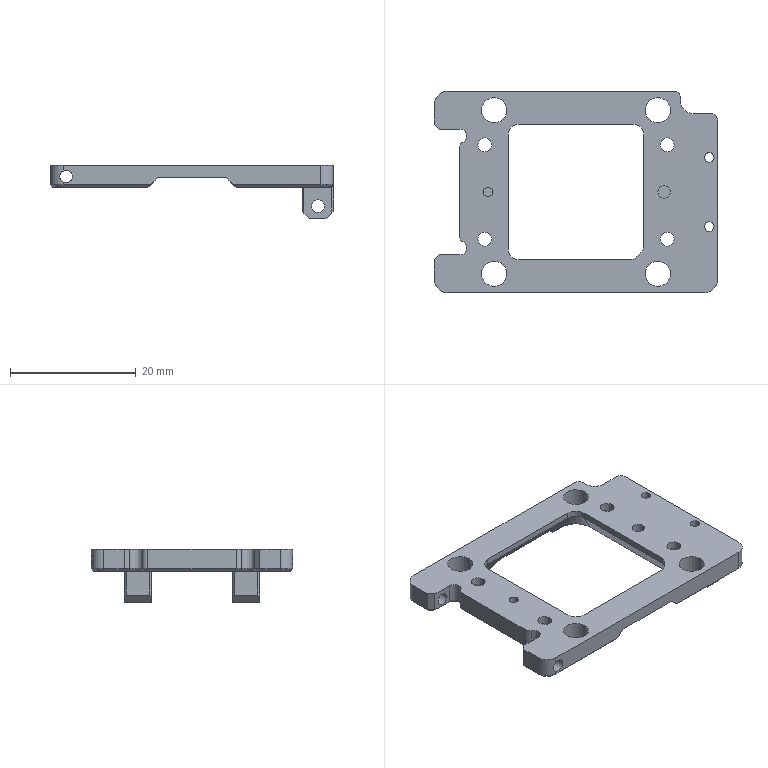NC program | NX | posted with a generic post | part box 45 x 32 x 8.5 mm
Lines 3037 to 3806 of 3806:
(CAVITY_MILL_COPY , TOOL : D1.5)
N6024 T19 M6
N6026 G54
N6028 G17 G0 G90 X-20.447 Y-8.95 B0. C0. S9500 M3
N6030 G43 Z30. H19
N6032 Z-0.146
N6034 G94 G3 X-19.733 Y-9.25 R1. F950.
N6036 G1 X-18.683
N6038 G2 X-18.483 Y-9.23 R0.76
N6040 G3 X-18.158 Y-8.974 R0.35
N6042 X-18.333 Y-8.592 R0.35
N6044 G2 X-19.055 Y-7.856 R1.75
N6046 G3 X-19.519 Y-7.41 R1.
N6048 G0 X-20.447 Y-8.95 Z-0.292
N6050 G3 X-19.733 Y-9.25 R1.
N6052 G1 X-18.683
N6054 G2 X-18.483 Y-9.23 R0.76
N6056 G3 X-18.158 Y-8.974 R0.35
N6058 X-18.333 Y-8.592 R0.35
N6060 G2 X-19.055 Y-7.856 R1.75
N6062 G3 X-19.519 Y-7.41 R1.
N6064 G0 X-20.447 Y-8.95 Z-0.438
N6066 G3 X-19.733 Y-9.25 R1.
N6068 G1 X-18.683
N6070 G2 X-18.483 Y-9.23 R0.76
N6072 G3 X-18.158 Y-8.974 R0.35
N6074 X-18.333 Y-8.592 R0.35
N6076 G2 X-19.055 Y-7.856 R1.75
N6078 G3 X-19.519 Y-7.41 R1.
N6080 G0 X-20.447 Y-8.95 Z-0.583
N6082 G3 X-19.733 Y-9.25 R1.
N6084 G1 X-18.683
N6086 G2 X-18.483 Y-9.23 R0.76
N6088 G3 X-18.158 Y-8.974 R0.35
N6090 X-18.333 Y-8.592 R0.35
N6092 G2 X-19.055 Y-7.856 R1.75
N6094 G3 X-19.519 Y-7.41 R1.
N6096 G0 X-20.447 Y-8.95 Z-0.729
N6098 G3 X-19.733 Y-9.25 R1.
N6100 G1 X-18.683
N6102 G2 X-18.483 Y-9.23 R0.76
N6104 G3 X-18.158 Y-8.974 R0.35
N6106 X-18.333 Y-8.592 R0.35
N6108 G2 X-19.055 Y-7.856 R1.75
N6110 G3 X-19.519 Y-7.41 R1.
N6112 G0 X-20.447 Y-8.95 Z-0.875
N6114 G3 X-19.733 Y-9.25 R1.
N6116 G1 X-18.683
N6118 G2 X-18.483 Y-9.23 R0.76
N6120 G3 X-18.158 Y-8.974 R0.35
N6122 X-18.333 Y-8.592 R0.35
N6124 G2 X-19.055 Y-7.856 R1.75
N6126 G3 X-19.519 Y-7.41 R1.
N6128 G0 X-20.447 Y-8.95 Z-1.021
N6130 G3 X-19.733 Y-9.25 R1.
N6132 G1 X-18.683
N6134 G2 X-18.483 Y-9.23 R0.76
N6136 G3 X-18.158 Y-8.974 R0.35
N6138 X-18.333 Y-8.592 R0.35
N6140 G2 X-19.055 Y-7.856 R1.75
N6142 G3 X-19.519 Y-7.41 R1.
N6144 G0 X-20.447 Y-8.95 Z-1.167
N6146 G3 X-19.733 Y-9.25 R1.
N6148 G1 X-18.683
N6150 G2 X-18.483 Y-9.23 R0.76
N6152 G3 X-18.158 Y-8.974 R0.35
N6154 X-18.333 Y-8.592 R0.35
N6156 G2 X-19.055 Y-7.856 R1.75
N6158 G3 X-19.519 Y-7.41 R1.
N6160 G0 X-20.447 Y-8.95 Z-1.313
N6162 G3 X-19.733 Y-9.25 R1.
N6164 G1 X-18.683
N6166 G2 X-18.483 Y-9.23 R0.76
N6168 G3 X-18.158 Y-8.974 R0.35
N6170 X-18.333 Y-8.592 R0.35
N6172 G2 X-19.055 Y-7.856 R1.75
N6174 G3 X-19.519 Y-7.41 R1.
N6176 G0 X-20.447 Y-8.95 Z-1.458
N6178 G3 X-19.733 Y-9.25 R1.
N6180 G1 X-18.683
N6182 G2 X-18.483 Y-9.23 R0.76
N6184 G3 X-18.158 Y-8.974 R0.35
N6186 X-18.333 Y-8.592 R0.35
N6188 G2 X-19.055 Y-7.856 R1.75
N6190 G3 X-19.519 Y-7.41 R1.
N6192 G0 X-20.447 Y-8.95 Z-1.604
N6194 G3 X-19.733 Y-9.25 R1.
N6196 G1 X-18.683
N6198 G2 X-18.483 Y-9.23 R0.76
N6200 G3 X-18.158 Y-8.974 R0.35
N6202 X-18.333 Y-8.592 R0.35
N6204 G2 X-19.055 Y-7.856 R1.75
N6206 G3 X-19.519 Y-7.41 R1.
N6208 G0 X-20.447 Y-8.95 Z-1.75
N6210 G3 X-19.733 Y-9.25 R1.
N6212 G1 X-18.683
N6214 G2 X-18.483 Y-9.23 R0.76
N6216 G3 X-18.158 Y-8.974 R0.35
N6218 X-18.333 Y-8.592 R0.35
N6220 G2 X-19.055 Y-7.856 R1.75
N6222 G3 X-19.519 Y-7.41 R1.
N6224 G0 X-20.447 Y-8.95 Z-1.896
N6226 G3 X-19.733 Y-9.25 R1.
N6228 G1 X-18.683
N6230 G2 X-18.483 Y-9.23 R0.76
N6232 G3 X-18.158 Y-8.974 R0.35
N6234 X-18.333 Y-8.592 R0.35
N6236 G2 X-19.055 Y-7.856 R1.75
N6238 G3 X-19.519 Y-7.41 R1.
N6240 G0 X-20.447 Y-8.95 Z-2.042
N6242 G3 X-19.733 Y-9.25 R1.
N6244 G1 X-18.683
N6246 G2 X-18.483 Y-9.23 R0.76
N6248 G3 X-18.158 Y-8.974 R0.35
N6250 X-18.333 Y-8.592 R0.35
N6252 G2 X-19.055 Y-7.856 R1.75
N6254 G3 X-19.519 Y-7.41 R1.
N6256 G0 X-20.447 Y-8.95 Z-2.188
N6258 G3 X-19.733 Y-9.25 R1.
N6260 G1 X-18.683
N6262 G2 X-18.483 Y-9.23 R0.76
N6264 G3 X-18.158 Y-8.974 R0.35
N6266 X-18.333 Y-8.592 R0.35
N6268 G2 X-19.055 Y-7.856 R1.75
N6270 G3 X-19.519 Y-7.41 R1.
N6272 G0 X-20.447 Y-8.95 Z-2.333
N6274 G3 X-19.733 Y-9.25 R1.
N6276 G1 X-18.683
N6278 G2 X-18.483 Y-9.23 R0.76
N6280 G3 X-18.158 Y-8.974 R0.35
N6282 X-18.333 Y-8.592 R0.35
N6284 G2 X-19.055 Y-7.856 R1.75
N6286 G3 X-19.519 Y-7.41 R1.
N6288 G0 X-20.447 Y-8.95 Z-2.479
N6290 G3 X-19.733 Y-9.25 R1.
N6292 G1 X-18.683
N6294 G2 X-18.483 Y-9.23 R0.76
N6296 G3 X-18.158 Y-8.974 R0.35
N6298 X-18.333 Y-8.592 R0.35
N6300 G2 X-19.055 Y-7.856 R1.75
N6302 G3 X-19.519 Y-7.41 R1.
N6304 G0 X-20.447 Y-8.95 Z-2.625
N6306 G3 X-19.733 Y-9.25 R1.
N6308 G1 X-18.683
N6310 G2 X-18.483 Y-9.23 R0.76
N6312 G3 X-18.158 Y-8.974 R0.35
N6314 X-18.333 Y-8.592 R0.35
N6316 G2 X-19.055 Y-7.856 R1.75
N6318 G3 X-19.519 Y-7.41 R1.
N6320 G0 X-20.447 Y-8.95 Z-2.771
N6322 G3 X-19.733 Y-9.25 R1.
N6324 G1 X-18.683
N6326 G2 X-18.483 Y-9.23 R0.76
N6328 G3 X-18.158 Y-8.974 R0.35
N6330 X-18.333 Y-8.592 R0.35
N6332 G2 X-19.055 Y-7.856 R1.75
N6334 G3 X-19.519 Y-7.41 R1.
N6336 G0 X-20.447 Y-8.95 Z-2.917
N6338 G3 X-19.733 Y-9.25 R1.
N6340 G1 X-18.683
N6342 G2 X-18.483 Y-9.23 R0.76
N6344 G3 X-18.158 Y-8.974 R0.35
N6346 X-18.333 Y-8.592 R0.35
N6348 G2 X-19.055 Y-7.856 R1.75
N6350 G3 X-19.519 Y-7.41 R1.
N6352 G0 X-20.447 Y-8.95 Z-3.063
N6354 G3 X-19.733 Y-9.25 R1.
N6356 G1 X-18.683
N6358 G2 X-18.483 Y-9.23 R0.76
N6360 G3 X-18.158 Y-8.974 R0.35
N6362 X-18.333 Y-8.592 R0.35
N6364 G2 X-19.055 Y-7.856 R1.75
N6366 G3 X-19.519 Y-7.41 R1.
N6368 G0 X-20.462 Y-8.95 Z-3.208
N6370 G3 X-19.748 Y-9.25 R1.
N6372 G1 X-18.683
N6374 G2 X-18.483 Y-9.23 R0.76
N6376 G3 X-18.158 Y-8.974 R0.35
N6378 X-18.333 Y-8.592 R0.35
N6380 G2 X-19.075 Y-7.816 R1.75
N6382 G3 X-19.527 Y-7.357 R1.
N6384 G0 X-20.462 Y-8.95 Z-3.354
N6386 G3 X-19.748 Y-9.25 R1.
N6388 G1 X-18.683
N6390 G2 X-18.483 Y-9.23 R0.76
N6392 G3 X-18.158 Y-8.974 R0.35
N6394 X-18.333 Y-8.592 R0.35
N6396 G2 X-19.075 Y-7.816 R1.75
N6398 G3 X-19.527 Y-7.357 R1.
N6400 G0 X-20.462 Y-8.95 Z-3.5
N6402 G3 X-19.748 Y-9.25 R1.
N6404 G1 X-18.683
N6406 G2 X-18.483 Y-9.23 R0.76
N6408 G3 X-18.158 Y-8.974 R0.35
N6410 X-18.333 Y-8.592 R0.35
N6412 G2 X-19.075 Y-7.816 R1.75
N6414 G3 X-19.527 Y-7.357 R1.
N6416 G0 Z30.
N6418 X-19.519 Y7.41
N6420 Z-0.146
N6422 G3 X-19.055 Y7.856 R1.
N6424 G2 X-18.333 Y8.592 R1.75
N6426 G3 X-18.158 Y8.974 R0.35
N6428 X-18.483 Y9.23 R0.331
N6430 G2 X-18.683 Y9.25 R0.76
N6432 G1 X-19.733
N6434 G3 X-20.447 Y8.95 R1.
N6436 G0 X-19.519 Y7.41 Z-0.292
N6438 G3 X-19.055 Y7.856 R1.
N6440 G2 X-18.333 Y8.592 R1.75
N6442 G3 X-18.158 Y8.974 R0.35
N6444 X-18.483 Y9.23 R0.331
N6446 G2 X-18.683 Y9.25 R0.76
N6448 G1 X-19.733
N6450 G3 X-20.447 Y8.95 R1.
N6452 G0 X-19.519 Y7.41 Z-0.438
N6454 G3 X-19.055 Y7.856 R1.
N6456 G2 X-18.333 Y8.592 R1.75
N6458 G3 X-18.158 Y8.974 R0.35
N6460 X-18.483 Y9.23 R0.331
N6462 G2 X-18.683 Y9.25 R0.76
N6464 G1 X-19.733
N6466 G3 X-20.447 Y8.95 R1.
N6468 G0 X-19.519 Y7.41 Z-0.583
N6470 G3 X-19.055 Y7.856 R1.
N6472 G2 X-18.333 Y8.592 R1.75
N6474 G3 X-18.158 Y8.974 R0.35
N6476 X-18.483 Y9.23 R0.331
N6478 G2 X-18.683 Y9.25 R0.76
N6480 G1 X-19.733
N6482 G3 X-20.447 Y8.95 R1.
N6484 G0 X-19.519 Y7.41 Z-0.729
N6486 G3 X-19.055 Y7.856 R1.
N6488 G2 X-18.333 Y8.592 R1.75
N6490 G3 X-18.158 Y8.974 R0.35
N6492 X-18.483 Y9.23 R0.331
N6494 G2 X-18.683 Y9.25 R0.76
N6496 G1 X-19.733
N6498 G3 X-20.447 Y8.95 R1.
N6500 G0 X-19.519 Y7.41 Z-0.875
N6502 G3 X-19.055 Y7.856 R1.
N6504 G2 X-18.333 Y8.592 R1.75
N6506 G3 X-18.158 Y8.974 R0.35
N6508 X-18.483 Y9.23 R0.331
N6510 G2 X-18.683 Y9.25 R0.76
N6512 G1 X-19.733
N6514 G3 X-20.447 Y8.95 R1.
N6516 G0 X-19.519 Y7.41 Z-1.021
N6518 G3 X-19.055 Y7.856 R1.
N6520 G2 X-18.333 Y8.592 R1.75
N6522 G3 X-18.158 Y8.974 R0.35
N6524 X-18.483 Y9.23 R0.331
N6526 G2 X-18.683 Y9.25 R0.76
N6528 G1 X-19.733
N6530 G3 X-20.447 Y8.95 R1.
N6532 G0 X-19.519 Y7.41 Z-1.167
N6534 G3 X-19.055 Y7.856 R1.
N6536 G2 X-18.333 Y8.592 R1.75
N6538 G3 X-18.158 Y8.974 R0.35
N6540 X-18.483 Y9.23 R0.331
N6542 G2 X-18.683 Y9.25 R0.76
N6544 G1 X-19.733
N6546 G3 X-20.447 Y8.95 R1.
N6548 G0 X-19.519 Y7.41 Z-1.313
N6550 G3 X-19.055 Y7.856 R1.
N6552 G2 X-18.333 Y8.592 R1.75
N6554 G3 X-18.158 Y8.974 R0.35
N6556 X-18.483 Y9.23 R0.331
N6558 G2 X-18.683 Y9.25 R0.76
N6560 G1 X-19.733
N6562 G3 X-20.447 Y8.95 R1.
N6564 G0 X-19.519 Y7.41 Z-1.458
N6566 G3 X-19.055 Y7.856 R1.
N6568 G2 X-18.333 Y8.592 R1.75
N6570 G3 X-18.158 Y8.974 R0.35
N6572 X-18.483 Y9.23 R0.331
N6574 G2 X-18.683 Y9.25 R0.76
N6576 G1 X-19.733
N6578 G3 X-20.447 Y8.95 R1.
N6580 G0 X-19.519 Y7.41 Z-1.604
N6582 G3 X-19.055 Y7.856 R1.
N6584 G2 X-18.333 Y8.592 R1.75
N6586 G3 X-18.158 Y8.974 R0.35
N6588 X-18.483 Y9.23 R0.331
N6590 G2 X-18.683 Y9.25 R0.76
N6592 G1 X-19.733
N6594 G3 X-20.447 Y8.95 R1.
N6596 G0 X-19.519 Y7.41 Z-1.75
N6598 G3 X-19.055 Y7.856 R1.
N6600 G2 X-18.333 Y8.592 R1.75
N6602 G3 X-18.158 Y8.974 R0.35
N6604 X-18.483 Y9.23 R0.331
N6606 G2 X-18.683 Y9.25 R0.76
N6608 G1 X-19.733
N6610 G3 X-20.447 Y8.95 R1.
N6612 G0 X-19.519 Y7.41 Z-1.896
N6614 G3 X-19.055 Y7.856 R1.
N6616 G2 X-18.333 Y8.592 R1.75
N6618 G3 X-18.158 Y8.974 R0.35
N6620 X-18.483 Y9.23 R0.331
N6622 G2 X-18.683 Y9.25 R0.76
N6624 G1 X-19.733
N6626 G3 X-20.447 Y8.95 R1.
N6628 G0 X-19.519 Y7.41 Z-2.042
N6630 G3 X-19.055 Y7.856 R1.
N6632 G2 X-18.333 Y8.592 R1.75
N6634 G3 X-18.158 Y8.974 R0.35
N6636 X-18.483 Y9.23 R0.331
N6638 G2 X-18.683 Y9.25 R0.76
N6640 G1 X-19.733
N6642 G3 X-20.447 Y8.95 R1.
N6644 G0 X-19.519 Y7.41 Z-2.188
N6646 G3 X-19.055 Y7.856 R1.
N6648 G2 X-18.333 Y8.592 R1.75
N6650 G3 X-18.158 Y8.974 R0.35
N6652 X-18.483 Y9.23 R0.331
N6654 G2 X-18.683 Y9.25 R0.76
N6656 G1 X-19.733
N6658 G3 X-20.447 Y8.95 R1.
N6660 G0 X-19.519 Y7.41 Z-2.333
N6662 G3 X-19.055 Y7.856 R1.
N6664 G2 X-18.333 Y8.592 R1.75
N6666 G3 X-18.158 Y8.974 R0.35
N6668 X-18.483 Y9.23 R0.331
N6670 G2 X-18.683 Y9.25 R0.76
N6672 G1 X-19.733
N6674 G3 X-20.447 Y8.95 R1.
N6676 G0 X-19.519 Y7.41 Z-2.479
N6678 G3 X-19.055 Y7.856 R1.
N6680 G2 X-18.333 Y8.592 R1.75
N6682 G3 X-18.158 Y8.974 R0.35
N6684 X-18.483 Y9.23 R0.331
N6686 G2 X-18.683 Y9.25 R0.76
N6688 G1 X-19.733
N6690 G3 X-20.447 Y8.95 R1.
N6692 G0 X-19.519 Y7.41 Z-2.625
N6694 G3 X-19.055 Y7.856 R1.
N6696 G2 X-18.333 Y8.592 R1.75
N6698 G3 X-18.158 Y8.974 R0.35
N6700 X-18.483 Y9.23 R0.331
N6702 G2 X-18.683 Y9.25 R0.76
N6704 G1 X-19.733
N6706 G3 X-20.447 Y8.95 R1.
N6708 G0 X-19.519 Y7.41 Z-2.771
N6710 G3 X-19.055 Y7.856 R1.
N6712 G2 X-18.333 Y8.592 R1.75
N6714 G3 X-18.158 Y8.974 R0.35
N6716 X-18.483 Y9.23 R0.331
N6718 G2 X-18.683 Y9.25 R0.76
N6720 G1 X-19.733
N6722 G3 X-20.447 Y8.95 R1.
N6724 G0 X-19.519 Y7.41 Z-2.917
N6726 G3 X-19.055 Y7.856 R1.
N6728 G2 X-18.333 Y8.592 R1.75
N6730 G3 X-18.158 Y8.974 R0.35
N6732 X-18.483 Y9.23 R0.331
N6734 G2 X-18.683 Y9.25 R0.76
N6736 G1 X-19.733
N6738 G3 X-20.447 Y8.95 R1.
N6740 G0 X-19.519 Y7.41 Z-3.063
N6742 G3 X-19.055 Y7.856 R1.
N6744 G2 X-18.333 Y8.592 R1.75
N6746 G3 X-18.158 Y8.974 R0.35
N6748 X-18.483 Y9.23 R0.331
N6750 G2 X-18.683 Y9.25 R0.76
N6752 G1 X-19.733
N6754 G3 X-20.447 Y8.95 R1.
N6756 G0 X-19.527 Y7.36 Z-3.208
N6758 G3 X-19.074 Y7.818 R1.
N6760 G2 X-18.333 Y8.592 R1.75
N6762 G3 X-18.158 Y8.974 R0.35
N6764 X-18.483 Y9.23 R0.331
N6766 G2 X-18.683 Y9.25 R0.76
N6768 G1 X-19.755
N6770 G3 X-20.469 Y8.95 R1.
N6772 G0 X-19.527 Y7.36 Z-3.354
N6774 G3 X-19.074 Y7.818 R1.
N6776 G2 X-18.333 Y8.592 R1.75
N6778 G3 X-18.158 Y8.974 R0.35
N6780 X-18.483 Y9.23 R0.331
N6782 G2 X-18.683 Y9.25 R0.76
N6784 G1 X-19.755
N6786 G3 X-20.469 Y8.95 R1.
N6788 G0 X-19.527 Y7.36 Z-3.5
N6790 G3 X-19.074 Y7.818 R1.
N6792 G2 X-18.333 Y8.592 R1.75
N6794 G3 X-18.158 Y8.974 R0.35
N6796 X-18.483 Y9.23 R0.331
N6798 G2 X-18.683 Y9.25 R0.76
N6800 G1 X-19.755
N6802 G3 X-20.469 Y8.95 R1.
N6804 G0 Z30.
N6806 M5
(HOLE_MILLING_COPY_COPY , TOOL : D1)
N6808 T21 M6
N6810 G54
N6812 G17 G0 G90 X-14. Y0. B0. C0. S9506 M3
N6814 G43 Z30. H21
N6816 Z0.5
N6818 G94 G3 X-13.905 Y-0.095 R0.095 F650.
N6820 X-13.81 Y0. R0.095
N6822 X-13.81 Y0. Z0.42 I-0.19 J0.
N6824 X-13.81 Y0. Z0.34 I-0.19 J0.
N6826 X-13.81 Y0. Z0.26 I-0.19 J0.
N6828 X-13.81 Y0. Z0.18 I-0.19 J0.
N6830 X-13.81 Y0. Z0.1 I-0.19 J0.
N6832 X-13.81 Y0. Z0.02 I-0.19 J0.
N6834 X-13.81 Y0. Z-0.06 I-0.19 J0.
N6836 X-13.81 Y0. Z-0.14 I-0.19 J0.
N6838 X-13.81 Y0. Z-0.22 I-0.19 J0.
N6840 X-13.81 Y0. Z-0.3 I-0.19 J0.
N6842 X-13.81 Y0. Z-0.38 I-0.19 J0.
N6844 X-13.81 Y0. Z-0.46 I-0.19 J0.
N6846 X-13.81 Y0. Z-0.54 I-0.19 J0.
N6848 X-13.81 Y0. Z-0.62 I-0.19 J0.
N6850 X-13.81 Y0. Z-0.7 I-0.19 J0.
N6852 X-13.81 Y0. Z-0.78 I-0.19 J0.
N6854 X-13.81 Y0. Z-0.86 I-0.19 J0.
N6856 X-13.81 Y0. Z-0.94 I-0.19 J0.
N6858 X-13.81 Y0. Z-1.02 I-0.19 J0.
N6860 X-13.81 Y0. Z-1.1 I-0.19 J0.
N6862 X-13.81 Y0. Z-1.18 I-0.19 J0.
N6864 X-13.81 Y0. Z-1.26 I-0.19 J0.
N6866 X-13.81 Y0. Z-1.34 I-0.19 J0.
N6868 X-13.81 Y0. Z-1.42 I-0.19 J0.
N6870 X-13.81 Y0. Z-1.5 I-0.19 J0.
N6872 X-13.81 Y0. Z-1.58 I-0.19 J0.
N6874 X-13.81 Y0. Z-1.66 I-0.19 J0.
N6876 X-13.81 Y0. Z-1.74 I-0.19 J0.
N6878 X-13.81 Y0. Z-1.82 I-0.19 J0.
N6880 X-13.81 Y0. Z-1.9 I-0.19 J0.
N6882 X-13.81 Y0. Z-1.98 I-0.19 J0.
N6884 X-13.81 Y0. Z-2.06 I-0.19 J0.
N6886 X-13.81 Y0. Z-2.14 I-0.19 J0.
N6888 X-13.81 Y0. Z-2.22 I-0.19 J0.
N6890 X-13.81 Y0. Z-2.3 I-0.19 J0.
N6892 X-13.81 Y0. Z-2.38 I-0.19 J0.
N6894 X-13.81 Y0. Z-2.46 I-0.19 J0.
N6896 X-14.19 Y0. Z-2.5 I-0.19 J0.
N6898 X-14. Y-0.19 R0.19
N6900 X-14.19 Y0. R-0.19
N6902 X-14.095 Y-0.095 R0.095
N6904 X-14. Y0. R0.095
N6906 G0 Z30.
N6908 X14.
N6910 Z0.5
N6912 G3 X14.22 Y-0.22 R0.22
N6914 X14.44 Y0. R0.22
N6916 X14.44 Y0. Z0.42 I-0.44 J0.
N6918 X14.44 Y0. Z0.34 I-0.44 J0.
N6920 X14.44 Y0. Z0.26 I-0.44 J0.
N6922 X14.44 Y0. Z0.18 I-0.44 J0.
N6924 X14.44 Y0. Z0.1 I-0.44 J0.
N6926 X14.44 Y0. Z0.02 I-0.44 J0.
N6928 X14.44 Y0. Z-0.06 I-0.44 J0.
N6930 X14.44 Y0. Z-0.14 I-0.44 J0.
N6932 X14.44 Y0. Z-0.22 I-0.44 J0.
N6934 X14.44 Y0. Z-0.3 I-0.44 J0.
N6936 X14.44 Y0. Z-0.38 I-0.44 J0.
N6938 X14.44 Y0. Z-0.46 I-0.44 J0.
N6940 X14.44 Y0. Z-0.54 I-0.44 J0.
N6942 X14.44 Y0. Z-0.62 I-0.44 J0.
N6944 X14.44 Y0. Z-0.7 I-0.44 J0.
N6946 X14.44 Y0. Z-0.78 I-0.44 J0.
N6948 X14.44 Y0. Z-0.86 I-0.44 J0.
N6950 X14.44 Y0. Z-0.94 I-0.44 J0.
N6952 X14.44 Y0. Z-1.02 I-0.44 J0.
N6954 X14.44 Y0. Z-1.1 I-0.44 J0.
N6956 X14.44 Y0. Z-1.18 I-0.44 J0.
N6958 X14.44 Y0. Z-1.26 I-0.44 J0.
N6960 X14.44 Y0. Z-1.34 I-0.44 J0.
N6962 X14.44 Y0. Z-1.42 I-0.44 J0.
N6964 X14.44 Y0. Z-1.5 I-0.44 J0.
N6966 X14.44 Y0. Z-1.58 I-0.44 J0.
N6968 X14.44 Y0. Z-1.66 I-0.44 J0.
N6970 X14.44 Y0. Z-1.74 I-0.44 J0.
N6972 X14.44 Y0. Z-1.82 I-0.44 J0.
N6974 X14.44 Y0. Z-1.9 I-0.44 J0.
N6976 X14.44 Y0. Z-1.98 I-0.44 J0.
N6978 X14.44 Y0. Z-2.06 I-0.44 J0.
N6980 X14.44 Y0. Z-2.14 I-0.44 J0.
N6982 X14.44 Y0. Z-2.22 I-0.44 J0.
N6984 X14.44 Y0. Z-2.3 I-0.44 J0.
N6986 X14.44 Y0. Z-2.38 I-0.44 J0.
N6988 X14.44 Y0. Z-2.46 I-0.44 J0.
N6990 X13.56 Y0. Z-2.5 I-0.44 J0.
N6992 X14. Y-0.44 R0.44
N6994 X13.56 Y0. R-0.44
N6996 X13.78 Y-0.22 R0.22
N6998 X14. Y0. R0.22
N7000 G0 Z30.
N7002 M5
(PLANAR_MILL , TOOL : D6A45)
N7004 T01 M6
N7006 G54
N7008 G17 G0 G90 X-13.866 Y-13.6 B0. C0. S9500 M3
N7010 G43 Z30. H1
N7012 Z0.5
N7014 G94 G1 Z-1. F1250.
N7016 G3 X-13. Y-14.1 R1.
N7018 X-11.9 Y-13. R1.1
N7020 X-13. Y-14.1 R-1.1
N7022 X-12.134 Y-13.6 R1.
N7024 G1 Z0.5
N7026 G0 Z30.
N7028 X-14.441 Y-7.5
N7030 Z0.5
N7032 G1 Z-1.
N7034 G3 X-14.7 Y-7.5 R0.5
N7036 X-14.5 Y-7.7 R0.2
N7038 X-14.7 Y-7.5 R-0.2
N7040 X-14.441 Y-7.5 R0.5
N7042 G1 Z0.5
N7044 G0 Z30.
N7046 Y7.5
N7048 Z0.5
N7050 G1 Z-1.
N7052 G3 X-14.7 Y7.5 R0.5
N7054 X-14.5 Y7.3 R0.2
N7056 X-14.7 Y7.5 R-0.2
N7058 X-14.441 Y7.5 R0.5
N7060 G1 Z0.5
N7062 G0 Z30.
N7064 X-12.134 Y13.6
N7066 Z0.5
N7068 G1 Z-1.
N7070 G3 X-13. Y14.1 R1.
N7072 X-14.1 Y13. R1.1
N7074 X-13. Y14.1 R-1.1
N7076 X-13.866 Y13.6 R1.
N7078 G1 Z0.5
N7080 G0 Z30.
N7082 X0.866 Y9.4
N7084 Z0.5
N7086 G1 Z-1.
N7088 G3 X0. Y9.9 R1.
N7090 G1 X-9.
N7092 G3 X-9.9 Y9. R0.9
N7094 G1 Y-9.
N7096 G3 X-9. Y-9.9 R0.9
N7098 G1 X8.379
N7100 G3 X9.015 Y-9.636 R0.9
N7102 G1 X9.636 Y-9.015
N7104 G3 X9.9 Y-8.379 R0.9
N7106 G1 Y9.
N7108 G3 X9. Y9.9 R0.9
N7110 G1 X0.
N7112 G3 X-0.866 Y9.4 R1.
N7114 G1 Z0.5
N7116 G0 Z30.
N7118 X-3.307 Y17.4
N7120 Z0.5
N7122 G1 Z-1.
N7124 G3 X-2.441 Y16.9 R1.
N7126 G1 X15.618
N7128 G2 X17.518 Y15. R1.9
N7130 G1 Y14.437
N7132 G3 X18.618 Y13.337 R1.1
N7134 G1 X21.5
N7136 G2 X23.4 Y11.437 R1.9
N7138 G1 Y-14.
N7140 G2 X20.5 Y-16.9 R2.9
N7142 G1 X-20.5
N7144 G2 X-23.4 Y-14. R2.9
N7146 G1 Y-10.8
N7148 G2 X-23.136 Y-10.164 R0.9
N7150 G1 X-22.336 Y-9.364
N7152 G2 X-21.7 Y-9.1 R0.9
N7154 G1 X-18.502
N7156 G3 X-18.405 Y-8.724 R0.2
N7158 G2 X-19.4 Y-7.053 R1.9
N7160 G1 Y7.053
N7162 G2 X-18.405 Y8.724 R1.9
N7164 G3 X-18.51 Y9.1 R0.2
N7166 G1 X-21.7
N7168 G2 X-22.336 Y9.364 R0.9
N7170 G1 X-23.136 Y10.164
N7172 G2 X-23.4 Y10.8 R0.9
N7174 G1 Y14.
N7176 G2 X-20.5 Y16.9 R2.9
N7178 G1 X-2.441
N7180 G3 X-1.575 Y17.4 R1.
N7182 G1 Z0.5
N7184 G0 Z30.
N7186 X12.134 Y-13.6
N7188 Z0.5
N7190 G1 Z-1.
N7192 G3 X13. Y-14.1 R1.
N7194 X14.1 Y-13. R1.1
N7196 X13. Y-14.1 R-1.1
N7198 X13.866 Y-13.6 R1.
N7200 G1 Z0.5
N7202 G0 Z30.
N7204 X14.441 Y-7.5
N7206 Z0.5
N7208 G1 Z-1.
N7210 G3 X14.7 Y-7.5 R0.5
N7212 X14.5 Y-7.3 R0.2
N7214 X14.7 Y-7.5 R-0.2
N7216 X14.441 Y-7.5 R0.5
N7218 G1 Z0.5
N7220 G0 Z30.
N7222 X14.09 Y-0.037
N7224 Z0.5
N7226 G1 Y0.079 Z0.469
N7228 X14.079 Y0.09 Z0.465
N7230 X13.921 Z0.422
N7232 X13.91 Y0.079 Z0.418
N7234 Y-0.079 Z0.376
N7236 X13.921 Y-0.09 Z0.372
N7238 X14.079 Z0.329
N7240 X14.09 Y-0.079 Z0.325
N7242 Y0.079 Z0.282
N7244 X14.079 Y0.09 Z0.278
N7246 X13.921 Z0.236
N7248 X13.91 Y0.079 Z0.232
N7250 Y-0.079 Z0.189
N7252 X13.921 Y-0.09 Z0.185
N7254 X14.079 Z0.143
N7256 X14.09 Y-0.079 Z0.139
N7258 Y0.079 Z0.096
N7260 X14.079 Y0.09 Z0.092
N7262 X13.921 Z0.05
N7264 X13.91 Y0.079 Z0.046
N7266 Y-0.079 Z0.003
N7268 X13.921 Y-0.09 Z-0.001
N7270 X14.079 Z-0.043
N7272 X14.09 Y-0.079 Z-0.047
N7274 Y0.079 Z-0.09
N7276 X14.079 Y0.09 Z-0.094
N7278 X13.921 Z-0.137
N7280 X13.91 Y0.079 Z-0.141
N7282 Y-0.079 Z-0.183
N7284 X13.921 Y-0.09 Z-0.187
N7286 X14.079 Z-0.23
N7288 X14.09 Y-0.079 Z-0.234
N7290 Y0.079 Z-0.276
N7292 X14.079 Y0.09 Z-0.28
N7294 X13.921 Z-0.323
N7296 X13.91 Y0.079 Z-0.327
N7298 Y-0.079 Z-0.369
N7300 X13.921 Y-0.09 Z-0.373
N7302 X14.079 Z-0.416
N7304 X14.09 Y-0.079 Z-0.42
N7306 Y0.079 Z-0.463
N7308 X14.079 Y0.09 Z-0.467
N7310 X13.921 Z-0.509
N7312 X13.91 Y0.079 Z-0.513
N7314 Y-0.079 Z-0.556
N7316 X13.921 Y-0.09 Z-0.56
N7318 X14.079 Z-0.602
N7320 X14.09 Y-0.079 Z-0.606
N7322 Y0.079 Z-0.649
N7324 X14.079 Y0.09 Z-0.653
N7326 X13.921 Z-0.695
N7328 X13.91 Y0.079 Z-0.699
N7330 Y-0.079 Z-0.742
N7332 X13.921 Y-0.09 Z-0.746
N7334 X14.079 Z-0.788
N7336 X14.09 Y-0.079 Z-0.792
N7338 Y0.079 Z-0.835
N7340 X14.079 Y0.09 Z-0.839
N7342 X13.921 Z-0.882
N7344 X13.91 Y0.079 Z-0.886
N7346 Y-0.079 Z-0.928
N7348 X13.921 Y-0.09 Z-0.932
N7350 X14.079 Z-0.975
N7352 X14.09 Y-0.079 Z-0.979
N7354 Y0. Z-1.
N7356 G3 X14. Y0.09 R0.09
N7358 X14.09 Y0. R-0.09
N7360 G1 Z0.5
N7362 G0 Z30.
N7364 X14.441 Y7.5
N7366 Z0.5
N7368 G1 Z-1.
N7370 G3 X14.7 Y7.5 R0.5
N7372 X14.5 Y7.7 R0.2
N7374 X14.7 Y7.5 R-0.2
N7376 X14.441 Y7.5 R0.5
N7378 G1 Z0.5
N7380 G0 Z30.
N7382 X13.866 Y13.6
N7384 Z0.5
N7386 G1 Z-1.
N7388 G3 X13. Y14.1 R1.
N7390 X11.9 Y13. R1.1
N7392 X13. Y14.1 R-1.1
N7394 X12.134 Y13.6 R1.
N7396 G1 Z0.5
N7398 G0 Z30.
N7400 M5
(CUTTERCOMP21. , TOOL : D1)
N7402 T21 M6
N7404 G54
N7406 G17 G0 G90 X-14. Y0. B0. C0. S9506 M3
N7408 G43 Z30. H21
N7410 Z0.5
N7412 G41 G94 G1 X-13.93 Y-0.072 F650. D21
N7414 X-13.868 Y-0.098
N7416 X-13.805 Y-0.066
N7418 X-13.79 Y0.
N7420 G3 X-13.79 Y0. Z0.35 I-0.21 J0.
N7422 X-13.79 Y0. Z0.2 I-0.21 J0.
N7424 X-13.79 Y0. Z0.05 I-0.21 J0.
N7426 X-13.79 Y0. Z-0.1 I-0.21 J0.
N7428 X-13.79 Y0. Z-0.25 I-0.21 J0.
N7430 X-13.79 Y0. Z-0.4 I-0.21 J0.
N7432 X-13.79 Y0. Z-0.55 I-0.21 J0.
N7434 X-13.79 Y0. Z-0.7 I-0.21 J0.
N7436 X-13.79 Y0. Z-0.85 I-0.21 J0.
N7438 X-13.79 Y0. Z-1. I-0.21 J0.
N7440 X-13.79 Y0. Z-1.15 I-0.21 J0.
N7442 X-13.79 Y0. Z-1.3 I-0.21 J0.
N7444 X-13.79 Y0. Z-1.45 I-0.21 J0.
N7446 X-13.79 Y0. Z-1.6 I-0.21 J0.
N7448 X-13.79 Y0. Z-1.75 I-0.21 J0.
N7450 X-13.79 Y0. Z-1.9 I-0.21 J0.
N7452 X-13.79 Y0. Z-2.05 I-0.21 J0.
N7454 X-13.79 Y0. Z-2.2 I-0.21 J0.
N7456 X-13.79 Y0. Z-2.35 I-0.21 J0.
N7458 X-13.79 Y0. Z-2.5 I-0.21 J0.
N7460 X-14. Y0.21 R0.21
N7462 X-13.79 Y0. R-0.21
N7464 G1 X-13.805 Y0.066
N7466 X-13.868 Y0.098
N7468 X-13.93 Y0.072
N7470 G40
N7472 X-14. Y0.
N7474 G0 Z30.
N7476 X14.
N7478 Z0.5
N7480 G41 G1 X14.026 Y-0.097
N7482 G3 X14.46 Y0. R0.228
N7484 X14.46 Y0. Z0.35 I-0.46 J0.
N7486 X14.46 Y0. Z0.2 I-0.46 J0.
N7488 X14.46 Y0. Z0.05 I-0.46 J0.
N7490 X14.46 Y0. Z-0.1 I-0.46 J0.
N7492 X14.46 Y0. Z-0.25 I-0.46 J0.
N7494 X14.46 Y0. Z-0.4 I-0.46 J0.
N7496 X14.46 Y0. Z-0.55 I-0.46 J0.
N7498 X14.46 Y0. Z-0.7 I-0.46 J0.
N7500 X14.46 Y0. Z-0.85 I-0.46 J0.
N7502 X14.46 Y0. Z-1. I-0.46 J0.
N7504 X14.46 Y0. Z-1.15 I-0.46 J0.
N7506 X14.46 Y0. Z-1.3 I-0.46 J0.
N7508 X14.46 Y0. Z-1.45 I-0.46 J0.
N7510 X14.46 Y0. Z-1.6 I-0.46 J0.
N7512 X14.46 Y0. Z-1.75 I-0.46 J0.
N7514 X14.46 Y0. Z-1.9 I-0.46 J0.
N7516 X14.46 Y0. Z-2.05 I-0.46 J0.
N7518 X14.46 Y0. Z-2.2 I-0.46 J0.
N7520 X14.46 Y0. Z-2.35 I-0.46 J0.
N7522 X14.46 Y0. Z-2.5 I-0.46 J0.
N7524 X14. Y0.46 R0.46
N7526 X14.46 Y0. R-0.46
N7528 X14.026 Y0.097 R0.228
N7530 G40
N7532 G1 X14. Y0.
N7534 G0 Z30.
N7536 M5
N7538 M2